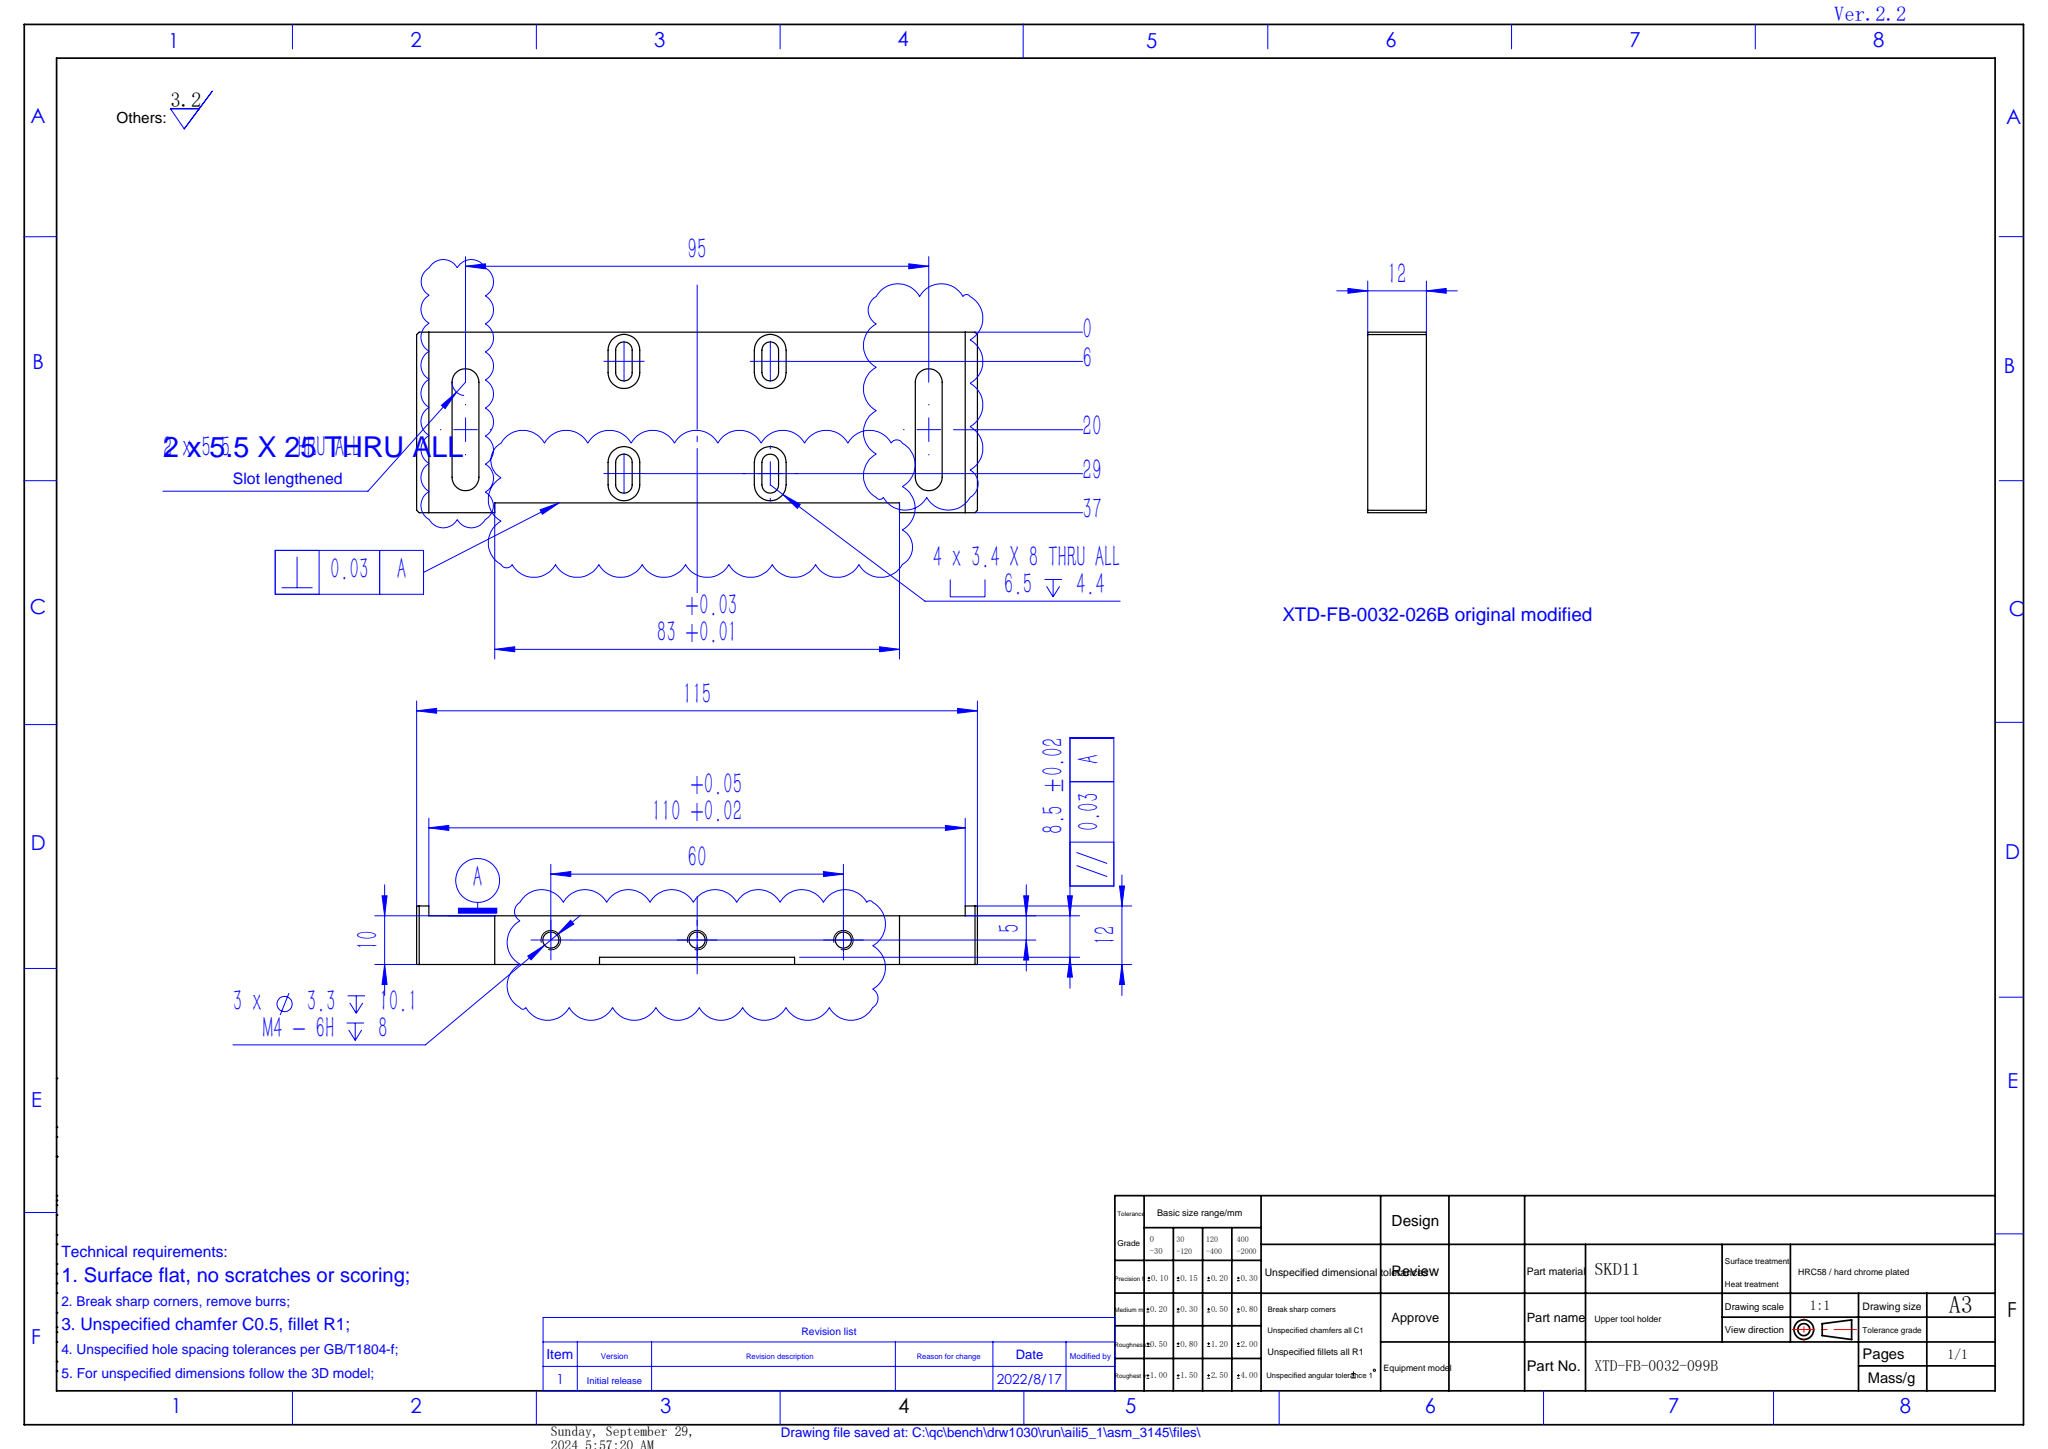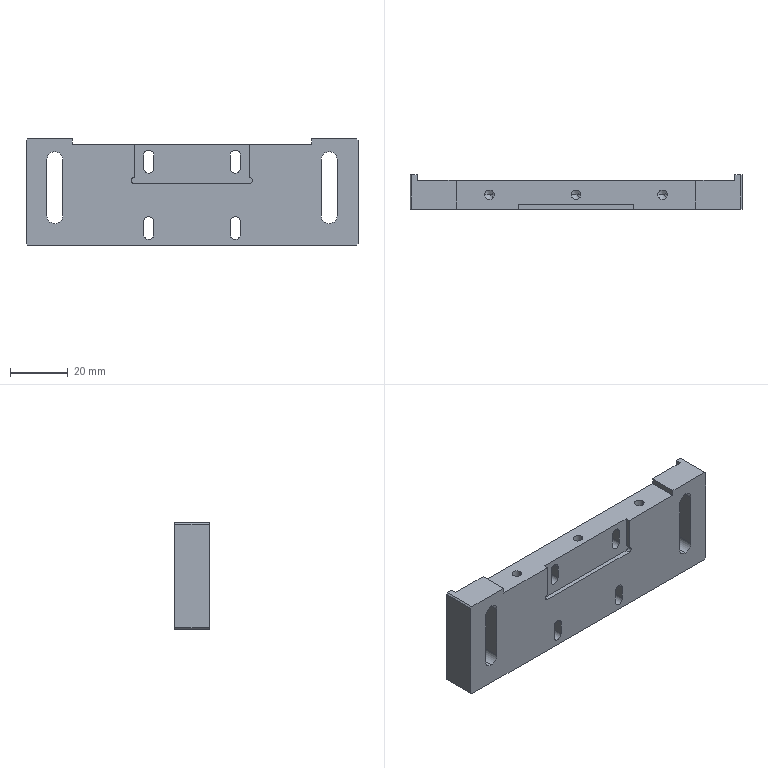Part | SolidWorks | features ICE 8, Cut 4, HoleWzd 4, Chamfer 1, Extrusion 1 | 1 solid | 91 faces | box 115 x 12 x 37 mm | volume 35962 mm3 | plane 46 | cylinder 39 | cone 6 | commonest cylinder face diameters 3.4 x12 6.5 x12 3.3 x6 5.5 x6 2 x3